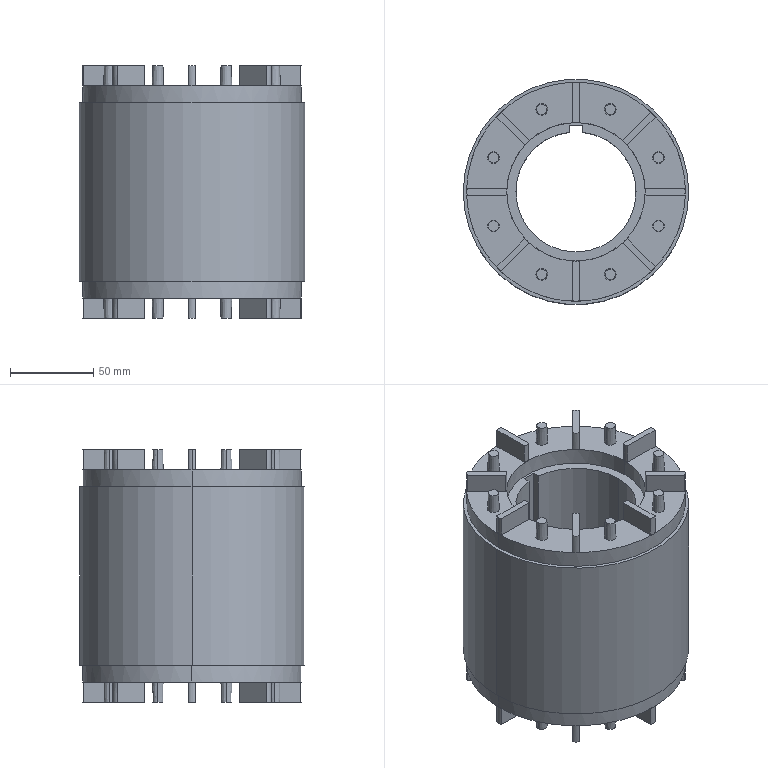Part | STEP file | Spindle Inner Ring | 1 solid | 170 faces | box 135 x 135 x 151 mm | volume 1278709 mm3 | plane 89 | cylinder 49 | cone 32 | commonest cylinder face diameters 8 x36 83 x4 131 x4 72 x3 135 x2